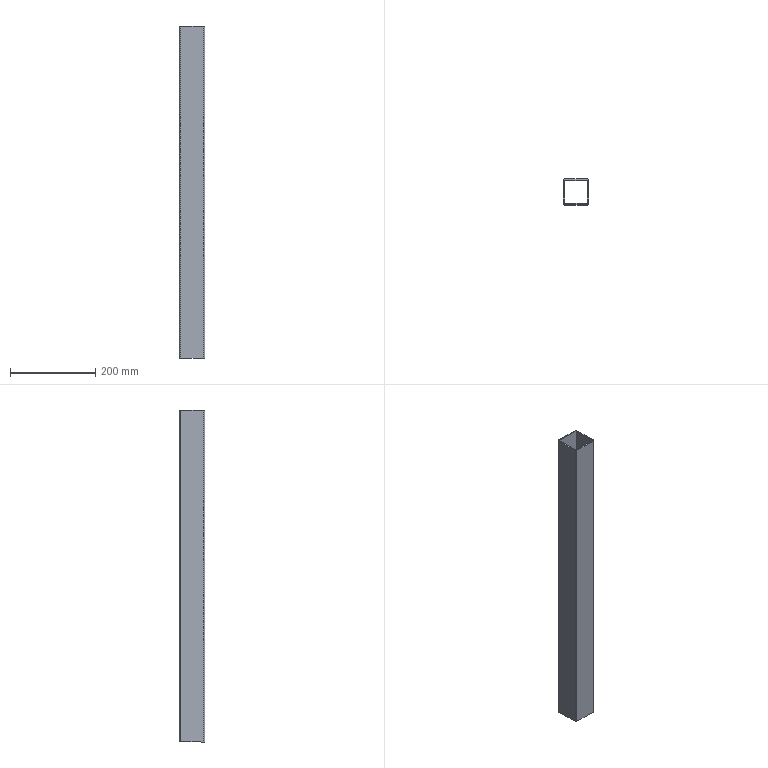Part | STEP file | X77-03108 | 1 solid | 14 faces | box 60 x 60 x 780 mm | volume 527494 mm3 | plane 10 | cylinder 4 | commonest cylinder face diameters 6 x4
STEP:
#1=CARTESIAN_POINT('',(0.,3.,780.));
#2=VERTEX_POINT('',#1);
#3=CARTESIAN_POINT('',(3.,0.,780.));
#4=VERTEX_POINT('',#3);
#5=CARTESIAN_POINT('',(3.,3.,780.));
#6=DIRECTION('',(0.,0.,1.));
#7=DIRECTION('',(1.,0.,0.));
#8=AXIS2_PLACEMENT_3D('',#5,#6,#7);
#9=CIRCLE('',#8,3.);
#10=EDGE_CURVE('',#2,#4,#9,.T.);
#11=ORIENTED_EDGE('',*,*,#10,.T.);
#12=CARTESIAN_POINT('',(57.,0.,780.));
#13=VERTEX_POINT('',#12);
#14=CARTESIAN_POINT('',(3.,0.,780.));
#15=DIRECTION('',(1.,0.,0.));
#16=VECTOR('',#15,1000.);
#17=LINE('',#14,#16);
#18=EDGE_CURVE('',#4,#13,#17,.T.);
#19=ORIENTED_EDGE('',*,*,#18,.T.);
#20=CARTESIAN_POINT('',(60.,3.,780.));
#21=VERTEX_POINT('',#20);
#22=CARTESIAN_POINT('',(57.,3.,780.));
#23=DIRECTION('',(0.,0.,1.));
#24=DIRECTION('',(1.,0.,0.));
#25=AXIS2_PLACEMENT_3D('',#22,#23,#24);
#26=CIRCLE('',#25,3.);
#27=EDGE_CURVE('',#13,#21,#26,.T.);
#28=ORIENTED_EDGE('',*,*,#27,.T.);
#29=CARTESIAN_POINT('',(60.,57.,780.));
#30=VERTEX_POINT('',#29);
#31=CARTESIAN_POINT('',(60.,3.,780.));
#32=DIRECTION('',(0.,1.,0.));
#33=VECTOR('',#32,1000.);
#34=LINE('',#31,#33);
#35=EDGE_CURVE('',#21,#30,#34,.T.);
#36=ORIENTED_EDGE('',*,*,#35,.T.);
#37=CARTESIAN_POINT('',(57.,60.,780.));
#38=VERTEX_POINT('',#37);
#39=CARTESIAN_POINT('',(57.,57.,780.));
#40=DIRECTION('',(0.,0.,1.));
#41=DIRECTION('',(1.,0.,0.));
#42=AXIS2_PLACEMENT_3D('',#39,#40,#41);
#43=CIRCLE('',#42,3.);
#44=EDGE_CURVE('',#30,#38,#43,.T.);
#45=ORIENTED_EDGE('',*,*,#44,.T.);
#46=CARTESIAN_POINT('',(3.,60.,780.));
#47=VERTEX_POINT('',#46);
#48=CARTESIAN_POINT('',(3.,60.,780.));
#49=DIRECTION('',(-1.,0.,0.));
#50=VECTOR('',#49,1000.);
#51=LINE('',#48,#50);
#52=EDGE_CURVE('',#38,#47,#51,.T.);
#53=ORIENTED_EDGE('',*,*,#52,.T.);
#54=CARTESIAN_POINT('',(0.,57.,780.));
#55=VERTEX_POINT('',#54);
#56=CARTESIAN_POINT('',(3.,57.,780.));
#57=DIRECTION('',(0.,0.,1.));
#58=DIRECTION('',(1.,0.,0.));
#59=AXIS2_PLACEMENT_3D('',#56,#57,#58);
#60=CIRCLE('',#59,3.);
#61=EDGE_CURVE('',#47,#55,#60,.T.);
#62=ORIENTED_EDGE('',*,*,#61,.T.);
#63=CARTESIAN_POINT('',(0.,3.,780.));
#64=DIRECTION('',(0.,-1.,0.));
#65=VECTOR('',#64,1000.);
#66=LINE('',#63,#65);
#67=EDGE_CURVE('',#55,#2,#66,.T.);
#68=ORIENTED_EDGE('',*,*,#67,.T.);
#69=EDGE_LOOP('',(#11,#19,#28,#36,#45,#53,#62,#68));
#70=FACE_OUTER_BOUND('',#69,.T.);
#71=CARTESIAN_POINT('',(3.,3.,780.));
#72=VERTEX_POINT('',#71);
#73=CARTESIAN_POINT('',(57.,3.,780.));
#74=VERTEX_POINT('',#73);
#75=CARTESIAN_POINT('',(3.,3.,780.));
#76=DIRECTION('',(1.,0.,0.));
#77=VECTOR('',#76,1000.);
#78=LINE('',#75,#77);
#79=EDGE_CURVE('',#72,#74,#78,.T.);
#80=ORIENTED_EDGE('',*,*,#79,.F.);
#81=CARTESIAN_POINT('',(3.,57.,780.));
#82=VERTEX_POINT('',#81);
#83=CARTESIAN_POINT('',(3.,3.,780.));
#84=DIRECTION('',(0.,-1.,0.));
#85=VECTOR('',#84,1000.);
#86=LINE('',#83,#85);
#87=EDGE_CURVE('',#82,#72,#86,.T.);
#88=ORIENTED_EDGE('',*,*,#87,.F.);
#89=CARTESIAN_POINT('',(57.,57.,780.));
#90=VERTEX_POINT('',#89);
#91=CARTESIAN_POINT('',(3.,57.,780.));
#92=DIRECTION('',(-1.,0.,0.));
#93=VECTOR('',#92,1000.);
#94=LINE('',#91,#93);
#95=EDGE_CURVE('',#90,#82,#94,.T.);
#96=ORIENTED_EDGE('',*,*,#95,.F.);
#97=CARTESIAN_POINT('',(57.,3.,780.));
#98=DIRECTION('',(0.,1.,0.));
#99=VECTOR('',#98,1000.);
#100=LINE('',#97,#99);
#101=EDGE_CURVE('',#74,#90,#100,.T.);
#102=ORIENTED_EDGE('',*,*,#101,.F.);
#103=EDGE_LOOP('',(#80,#88,#96,#102));
#104=FACE_BOUND('',#103,.T.);
#105=CARTESIAN_POINT('',(3.,3.,780.));
#106=DIRECTION('',(0.,0.,1.));
#107=DIRECTION('',(1.,0.,0.));
#108=AXIS2_PLACEMENT_3D('',#105,#106,#107);
#109=PLANE('',#108);
#110=ADVANCED_FACE('',(#70,#104),#109,.T.);
#111=CARTESIAN_POINT('',(0.,3.,0.));
#112=VERTEX_POINT('',#111);
#113=CARTESIAN_POINT('',(3.,0.,0.));
#114=VERTEX_POINT('',#113);
#115=CARTESIAN_POINT('',(3.,3.,0.));
#116=DIRECTION('',(0.,0.,1.));
#117=DIRECTION('',(1.,0.,0.));
#118=AXIS2_PLACEMENT_3D('',#115,#116,#117);
#119=CIRCLE('',#118,3.);
#120=EDGE_CURVE('',#112,#114,#119,.T.);
#121=ORIENTED_EDGE('',*,*,#120,.F.);
#122=CARTESIAN_POINT('',(0.,57.,0.));
#123=VERTEX_POINT('',#122);
#124=CARTESIAN_POINT('',(0.,3.,0.));
#125=DIRECTION('',(0.,-1.,0.));
#126=VECTOR('',#125,1000.);
#127=LINE('',#124,#126);
#128=EDGE_CURVE('',#123,#112,#127,.T.);
#129=ORIENTED_EDGE('',*,*,#128,.F.);
#130=CARTESIAN_POINT('',(3.,60.,0.));
#131=VERTEX_POINT('',#130);
#132=CARTESIAN_POINT('',(3.,57.,0.));
#133=DIRECTION('',(0.,0.,1.));
#134=DIRECTION('',(1.,0.,0.));
#135=AXIS2_PLACEMENT_3D('',#132,#133,#134);
#136=CIRCLE('',#135,3.);
#137=EDGE_CURVE('',#131,#123,#136,.T.);
#138=ORIENTED_EDGE('',*,*,#137,.F.);
#139=CARTESIAN_POINT('',(57.,60.,0.));
#140=VERTEX_POINT('',#139);
#141=CARTESIAN_POINT('',(3.,60.,0.));
#142=DIRECTION('',(-1.,0.,0.));
#143=VECTOR('',#142,1000.);
#144=LINE('',#141,#143);
#145=EDGE_CURVE('',#140,#131,#144,.T.);
#146=ORIENTED_EDGE('',*,*,#145,.F.);
#147=CARTESIAN_POINT('',(60.,57.,0.));
#148=VERTEX_POINT('',#147);
#149=CARTESIAN_POINT('',(57.,57.,0.));
#150=DIRECTION('',(0.,0.,1.));
#151=DIRECTION('',(1.,0.,0.));
#152=AXIS2_PLACEMENT_3D('',#149,#150,#151);
#153=CIRCLE('',#152,3.);
#154=EDGE_CURVE('',#148,#140,#153,.T.);
#155=ORIENTED_EDGE('',*,*,#154,.F.);
#156=CARTESIAN_POINT('',(60.,3.,0.));
#157=VERTEX_POINT('',#156);
#158=CARTESIAN_POINT('',(60.,3.,0.));
#159=DIRECTION('',(0.,1.,0.));
#160=VECTOR('',#159,1000.);
#161=LINE('',#158,#160);
#162=EDGE_CURVE('',#157,#148,#161,.T.);
#163=ORIENTED_EDGE('',*,*,#162,.F.);
#164=CARTESIAN_POINT('',(57.,0.,0.));
#165=VERTEX_POINT('',#164);
#166=CARTESIAN_POINT('',(57.,3.,0.));
#167=DIRECTION('',(0.,0.,1.));
#168=DIRECTION('',(1.,0.,0.));
#169=AXIS2_PLACEMENT_3D('',#166,#167,#168);
#170=CIRCLE('',#169,3.);
#171=EDGE_CURVE('',#165,#157,#170,.T.);
#172=ORIENTED_EDGE('',*,*,#171,.F.);
#173=CARTESIAN_POINT('',(3.,0.,0.));
#174=DIRECTION('',(1.,0.,0.));
#175=VECTOR('',#174,1000.);
#176=LINE('',#173,#175);
#177=EDGE_CURVE('',#114,#165,#176,.T.);
#178=ORIENTED_EDGE('',*,*,#177,.F.);
#179=EDGE_LOOP('',(#121,#129,#138,#146,#155,#163,#172,#178));
#180=FACE_OUTER_BOUND('',#179,.T.);
#181=CARTESIAN_POINT('',(3.,57.,0.));
#182=VERTEX_POINT('',#181);
#183=CARTESIAN_POINT('',(3.,3.,0.));
#184=VERTEX_POINT('',#183);
#185=CARTESIAN_POINT('',(3.,3.,0.));
#186=DIRECTION('',(0.,-1.,0.));
#187=VECTOR('',#186,1000.);
#188=LINE('',#185,#187);
#189=EDGE_CURVE('',#182,#184,#188,.T.);
#190=ORIENTED_EDGE('',*,*,#189,.T.);
#191=CARTESIAN_POINT('',(57.,3.,0.));
#192=VERTEX_POINT('',#191);
#193=CARTESIAN_POINT('',(3.,3.,0.));
#194=DIRECTION('',(1.,0.,0.));
#195=VECTOR('',#194,1000.);
#196=LINE('',#193,#195);
#197=EDGE_CURVE('',#184,#192,#196,.T.);
#198=ORIENTED_EDGE('',*,*,#197,.T.);
#199=CARTESIAN_POINT('',(57.,57.,0.));
#200=VERTEX_POINT('',#199);
#201=CARTESIAN_POINT('',(57.,3.,0.));
#202=DIRECTION('',(0.,1.,0.));
#203=VECTOR('',#202,1000.);
#204=LINE('',#201,#203);
#205=EDGE_CURVE('',#192,#200,#204,.T.);
#206=ORIENTED_EDGE('',*,*,#205,.T.);
#207=CARTESIAN_POINT('',(3.,57.,0.));
#208=DIRECTION('',(-1.,0.,0.));
#209=VECTOR('',#208,1000.);
#210=LINE('',#207,#209);
#211=EDGE_CURVE('',#200,#182,#210,.T.);
#212=ORIENTED_EDGE('',*,*,#211,.T.);
#213=EDGE_LOOP('',(#190,#198,#206,#212));
#214=FACE_BOUND('',#213,.T.);
#215=CARTESIAN_POINT('',(3.,3.,0.));
#216=DIRECTION('',(0.,0.,1.));
#217=DIRECTION('',(1.,0.,0.));
#218=AXIS2_PLACEMENT_3D('',#215,#216,#217);
#219=PLANE('',#218);
#220=ADVANCED_FACE('',(#180,#214),#219,.F.);
#221=ORIENTED_EDGE('',*,*,#120,.T.);
#222=CARTESIAN_POINT('',(3.,0.,780.));
#223=DIRECTION('',(0.,0.,-1.));
#224=VECTOR('',#223,1000.);
#225=LINE('',#222,#224);
#226=EDGE_CURVE('',#4,#114,#225,.T.);
#227=ORIENTED_EDGE('',*,*,#226,.F.);
#228=ORIENTED_EDGE('',*,*,#10,.F.);
#229=CARTESIAN_POINT('',(0.,3.,780.));
#230=DIRECTION('',(0.,0.,-1.));
#231=VECTOR('',#230,1000.);
#232=LINE('',#229,#231);
#233=EDGE_CURVE('',#2,#112,#232,.T.);
#234=ORIENTED_EDGE('',*,*,#233,.T.);
#235=EDGE_LOOP('',(#221,#227,#228,#234));
#236=FACE_OUTER_BOUND('',#235,.T.);
#237=CARTESIAN_POINT('',(3.,3.,780.));
#238=DIRECTION('',(0.,0.,-1.));
#239=DIRECTION('',(-1.,0.,0.));
#240=AXIS2_PLACEMENT_3D('',#237,#238,#239);
#241=CYLINDRICAL_SURFACE('',#240,3.);
#242=ADVANCED_FACE('',(#236),#241,.T.);
#243=ORIENTED_EDGE('',*,*,#177,.T.);
#244=CARTESIAN_POINT('',(57.,0.,780.));
#245=DIRECTION('',(0.,0.,-1.));
#246=VECTOR('',#245,1000.);
#247=LINE('',#244,#246);
#248=EDGE_CURVE('',#13,#165,#247,.T.);
#249=ORIENTED_EDGE('',*,*,#248,.F.);
#250=ORIENTED_EDGE('',*,*,#18,.F.);
#251=ORIENTED_EDGE('',*,*,#226,.T.);
#252=EDGE_LOOP('',(#243,#249,#250,#251));
#253=FACE_OUTER_BOUND('',#252,.T.);
#254=CARTESIAN_POINT('',(3.,0.,780.));
#255=DIRECTION('',(0.,1.,0.));
#256=DIRECTION('',(0.,0.,1.));
#257=AXIS2_PLACEMENT_3D('',#254,#255,#256);
#258=PLANE('',#257);
#259=ADVANCED_FACE('',(#253),#258,.F.);
#260=ORIENTED_EDGE('',*,*,#171,.T.);
#261=CARTESIAN_POINT('',(60.,3.,780.));
#262=DIRECTION('',(0.,0.,-1.));
#263=VECTOR('',#262,1000.);
#264=LINE('',#261,#263);
#265=EDGE_CURVE('',#21,#157,#264,.T.);
#266=ORIENTED_EDGE('',*,*,#265,.F.);
#267=ORIENTED_EDGE('',*,*,#27,.F.);
#268=ORIENTED_EDGE('',*,*,#248,.T.);
#269=EDGE_LOOP('',(#260,#266,#267,#268));
#270=FACE_OUTER_BOUND('',#269,.T.);
#271=CARTESIAN_POINT('',(57.,3.,780.));
#272=DIRECTION('',(0.,0.,-1.));
#273=DIRECTION('',(-1.,0.,0.));
#274=AXIS2_PLACEMENT_3D('',#271,#272,#273);
#275=CYLINDRICAL_SURFACE('',#274,3.);
#276=ADVANCED_FACE('',(#270),#275,.T.);
#277=ORIENTED_EDGE('',*,*,#162,.T.);
#278=CARTESIAN_POINT('',(60.,57.,780.));
#279=DIRECTION('',(0.,0.,-1.));
#280=VECTOR('',#279,1000.);
#281=LINE('',#278,#280);
#282=EDGE_CURVE('',#30,#148,#281,.T.);
#283=ORIENTED_EDGE('',*,*,#282,.F.);
#284=ORIENTED_EDGE('',*,*,#35,.F.);
#285=ORIENTED_EDGE('',*,*,#265,.T.);
#286=EDGE_LOOP('',(#277,#283,#284,#285));
#287=FACE_OUTER_BOUND('',#286,.T.);
#288=CARTESIAN_POINT('',(60.,3.,780.));
#289=DIRECTION('',(-1.,0.,0.));
#290=DIRECTION('',(0.,0.,1.));
#291=AXIS2_PLACEMENT_3D('',#288,#289,#290);
#292=PLANE('',#291);
#293=ADVANCED_FACE('',(#287),#292,.F.);
#294=ORIENTED_EDGE('',*,*,#154,.T.);
#295=CARTESIAN_POINT('',(57.,60.,780.));
#296=DIRECTION('',(0.,0.,-1.));
#297=VECTOR('',#296,1000.);
#298=LINE('',#295,#297);
#299=EDGE_CURVE('',#38,#140,#298,.T.);
#300=ORIENTED_EDGE('',*,*,#299,.F.);
#301=ORIENTED_EDGE('',*,*,#44,.F.);
#302=ORIENTED_EDGE('',*,*,#282,.T.);
#303=EDGE_LOOP('',(#294,#300,#301,#302));
#304=FACE_OUTER_BOUND('',#303,.T.);
#305=CARTESIAN_POINT('',(57.,57.,780.));
#306=DIRECTION('',(0.,0.,-1.));
#307=DIRECTION('',(-1.,0.,0.));
#308=AXIS2_PLACEMENT_3D('',#305,#306,#307);
#309=CYLINDRICAL_SURFACE('',#308,3.);
#310=ADVANCED_FACE('',(#304),#309,.T.);
#311=ORIENTED_EDGE('',*,*,#145,.T.);
#312=CARTESIAN_POINT('',(3.,60.,780.));
#313=DIRECTION('',(0.,0.,-1.));
#314=VECTOR('',#313,1000.);
#315=LINE('',#312,#314);
#316=EDGE_CURVE('',#47,#131,#315,.T.);
#317=ORIENTED_EDGE('',*,*,#316,.F.);
#318=ORIENTED_EDGE('',*,*,#52,.F.);
#319=ORIENTED_EDGE('',*,*,#299,.T.);
#320=EDGE_LOOP('',(#311,#317,#318,#319));
#321=FACE_OUTER_BOUND('',#320,.T.);
#322=CARTESIAN_POINT('',(3.,60.,780.));
#323=DIRECTION('',(0.,-1.,0.));
#324=DIRECTION('',(0.,0.,-1.));
#325=AXIS2_PLACEMENT_3D('',#322,#323,#324);
#326=PLANE('',#325);
#327=ADVANCED_FACE('',(#321),#326,.F.);
#328=ORIENTED_EDGE('',*,*,#137,.T.);
#329=CARTESIAN_POINT('',(0.,57.,780.));
#330=DIRECTION('',(0.,0.,-1.));
#331=VECTOR('',#330,1000.);
#332=LINE('',#329,#331);
#333=EDGE_CURVE('',#55,#123,#332,.T.);
#334=ORIENTED_EDGE('',*,*,#333,.F.);
#335=ORIENTED_EDGE('',*,*,#61,.F.);
#336=ORIENTED_EDGE('',*,*,#316,.T.);
#337=EDGE_LOOP('',(#328,#334,#335,#336));
#338=FACE_OUTER_BOUND('',#337,.T.);
#339=CARTESIAN_POINT('',(3.,57.,780.));
#340=DIRECTION('',(0.,0.,-1.));
#341=DIRECTION('',(-1.,0.,0.));
#342=AXIS2_PLACEMENT_3D('',#339,#340,#341);
#343=CYLINDRICAL_SURFACE('',#342,3.);
#344=ADVANCED_FACE('',(#338),#343,.T.);
#345=ORIENTED_EDGE('',*,*,#128,.T.);
#346=ORIENTED_EDGE('',*,*,#233,.F.);
#347=ORIENTED_EDGE('',*,*,#67,.F.);
#348=ORIENTED_EDGE('',*,*,#333,.T.);
#349=EDGE_LOOP('',(#345,#346,#347,#348));
#350=FACE_OUTER_BOUND('',#349,.T.);
#351=CARTESIAN_POINT('',(0.,3.,780.));
#352=DIRECTION('',(1.,0.,0.));
#353=DIRECTION('',(0.,0.,-1.));
#354=AXIS2_PLACEMENT_3D('',#351,#352,#353);
#355=PLANE('',#354);
#356=ADVANCED_FACE('',(#350),#355,.F.);
#357=ORIENTED_EDGE('',*,*,#189,.F.);
#358=CARTESIAN_POINT('',(3.,57.,780.));
#359=DIRECTION('',(0.,0.,-1.));
#360=VECTOR('',#359,1000.);
#361=LINE('',#358,#360);
#362=EDGE_CURVE('',#82,#182,#361,.T.);
#363=ORIENTED_EDGE('',*,*,#362,.F.);
#364=ORIENTED_EDGE('',*,*,#87,.T.);
#365=CARTESIAN_POINT('',(3.,3.,780.));
#366=DIRECTION('',(0.,0.,-1.));
#367=VECTOR('',#366,1000.);
#368=LINE('',#365,#367);
#369=EDGE_CURVE('',#72,#184,#368,.T.);
#370=ORIENTED_EDGE('',*,*,#369,.T.);
#371=EDGE_LOOP('',(#357,#363,#364,#370));
#372=FACE_OUTER_BOUND('',#371,.T.);
#373=CARTESIAN_POINT('',(3.,3.,780.));
#374=DIRECTION('',(1.,0.,0.));
#375=DIRECTION('',(0.,0.,-1.));
#376=AXIS2_PLACEMENT_3D('',#373,#374,#375);
#377=PLANE('',#376);
#378=ADVANCED_FACE('',(#372),#377,.T.);
#379=ORIENTED_EDGE('',*,*,#197,.F.);
#380=ORIENTED_EDGE('',*,*,#369,.F.);
#381=ORIENTED_EDGE('',*,*,#79,.T.);
#382=CARTESIAN_POINT('',(57.,3.,780.));
#383=DIRECTION('',(0.,0.,-1.));
#384=VECTOR('',#383,1000.);
#385=LINE('',#382,#384);
#386=EDGE_CURVE('',#74,#192,#385,.T.);
#387=ORIENTED_EDGE('',*,*,#386,.T.);
#388=EDGE_LOOP('',(#379,#380,#381,#387));
#389=FACE_OUTER_BOUND('',#388,.T.);
#390=CARTESIAN_POINT('',(3.,3.,780.));
#391=DIRECTION('',(0.,1.,0.));
#392=DIRECTION('',(0.,0.,1.));
#393=AXIS2_PLACEMENT_3D('',#390,#391,#392);
#394=PLANE('',#393);
#395=ADVANCED_FACE('',(#389),#394,.T.);
#396=ORIENTED_EDGE('',*,*,#205,.F.);
#397=ORIENTED_EDGE('',*,*,#386,.F.);
#398=ORIENTED_EDGE('',*,*,#101,.T.);
#399=CARTESIAN_POINT('',(57.,57.,780.));
#400=DIRECTION('',(0.,0.,-1.));
#401=VECTOR('',#400,1000.);
#402=LINE('',#399,#401);
#403=EDGE_CURVE('',#90,#200,#402,.T.);
#404=ORIENTED_EDGE('',*,*,#403,.T.);
#405=EDGE_LOOP('',(#396,#397,#398,#404));
#406=FACE_OUTER_BOUND('',#405,.T.);
#407=CARTESIAN_POINT('',(57.,3.,780.));
#408=DIRECTION('',(-1.,0.,0.));
#409=DIRECTION('',(0.,0.,1.));
#410=AXIS2_PLACEMENT_3D('',#407,#408,#409);
#411=PLANE('',#410);
#412=ADVANCED_FACE('',(#406),#411,.T.);
#413=ORIENTED_EDGE('',*,*,#211,.F.);
#414=ORIENTED_EDGE('',*,*,#403,.F.);
#415=ORIENTED_EDGE('',*,*,#95,.T.);
#416=ORIENTED_EDGE('',*,*,#362,.T.);
#417=EDGE_LOOP('',(#413,#414,#415,#416));
#418=FACE_OUTER_BOUND('',#417,.T.);
#419=CARTESIAN_POINT('',(3.,57.,780.));
#420=DIRECTION('',(0.,-1.,0.));
#421=DIRECTION('',(0.,0.,-1.));
#422=AXIS2_PLACEMENT_3D('',#419,#420,#421);
#423=PLANE('',#422);
#424=ADVANCED_FACE('',(#418),#423,.T.);
#425=CLOSED_SHELL('',(#110,#220,#242,#259,#276,#293,#310,#327,#344,#356,#378,#395,#412,#424));
#426=MANIFOLD_SOLID_BREP('',#425);
#427=CARTESIAN_POINT('',(0.,0.,0.));
#428=DIRECTION('',(0.,0.,1.));
#429=DIRECTION('',(1.,0.,0.));
#430=AXIS2_PLACEMENT_3D('',#427,#428,#429);
#431=(LENGTH_UNIT()NAMED_UNIT(*)SI_UNIT(.MILLI.,.METRE.));
#432=UNCERTAINTY_MEASURE_WITH_UNIT(LENGTH_MEASURE(0.00001),#431,'','');
#433=(NAMED_UNIT(*)PLANE_ANGLE_UNIT()SI_UNIT($,.RADIAN.));
#434=(NAMED_UNIT(*)SI_UNIT($,.STERADIAN.)SOLID_ANGLE_UNIT());
#435=(GEOMETRIC_REPRESENTATION_CONTEXT(3)GLOBAL_UNCERTAINTY_ASSIGNED_CONTEXT((#432))GLOBAL_UNIT_ASSIGNED_CONTEXT((#431,#433,#434))REPRESENTATION_CONTEXT('',''));
#436=ADVANCED_BREP_SHAPE_REPRESENTATION('',(#426,#430),#435);